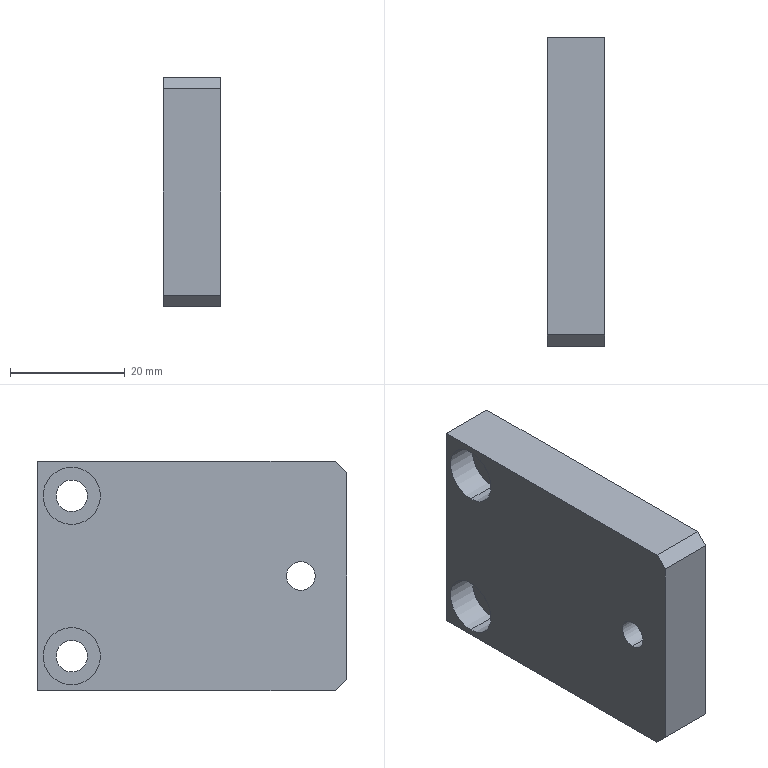Part | STEP file | PN_0015 | 1 solid | 20 faces | box 10 x 54 x 40 mm | volume 20297 mm3 | cylinder 10 | plane 10 | commonest cylinder face diameters 5.5 x4 10 x4 5 x2